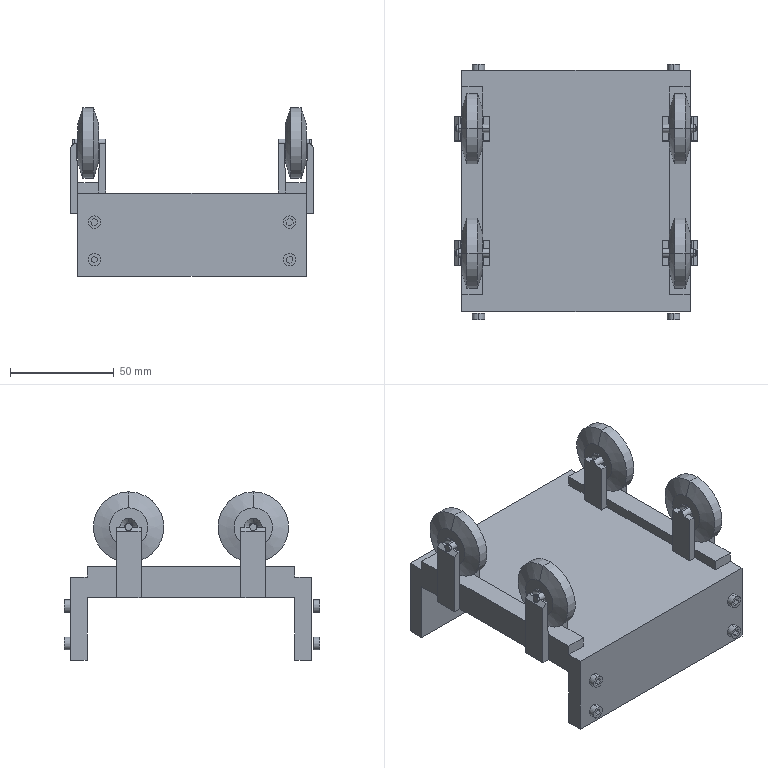Part | SolidWorks | features ICE 7, LPattern 4, Chamfer 1, Extrusion 1, MirrorPattern 1, Revolution 1 | 7 solids | 250 faces | box 117 x 123 x 81 mm | volume 229130 mm3 | plane 166 | cylinder 52 | cone 32 | commonest cylinder face diameters 4 x16 6 x16 3.407 x12 34 x8